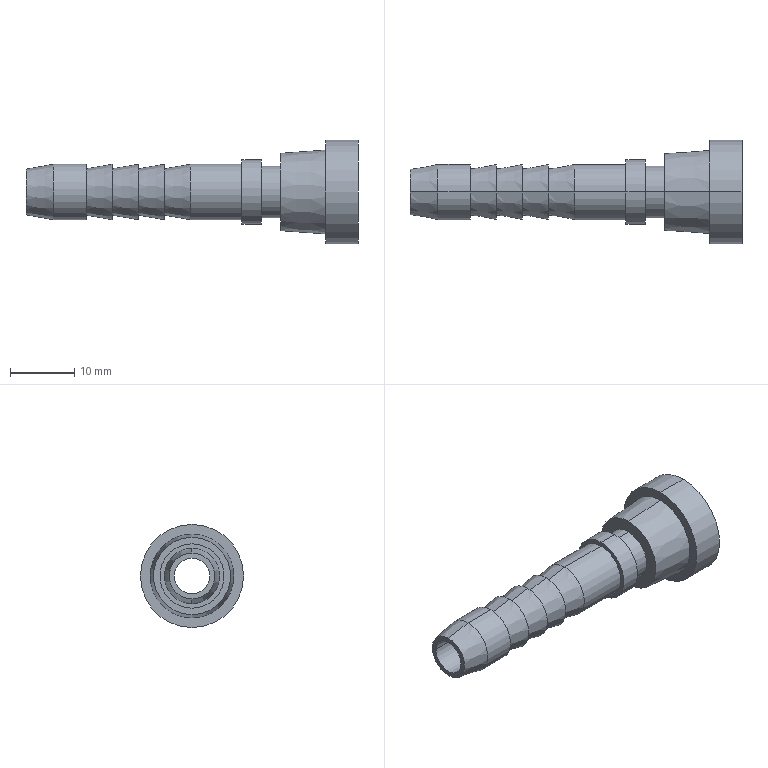Part | SolidWorks | features BaseBody 1 | 1 solid | 34 faces | box 51.5 x 16 x 16 mm | volume 2788 mm3 | cone 12 | cylinder 12 | plane 10 | commonest cylinder face diameters 8.6 x4 5.5 x2 8 x2 10 x2 16 x2
STEP:
#1=CARTESIAN_POINT('',(-12.,0.,-6.));
#2=VERTEX_POINT('',#1);
#3=CARTESIAN_POINT('',(-12.,0.,6.));
#4=VERTEX_POINT('',#3);
#5=CARTESIAN_POINT('',(-12.,0.,0.));
#6=DIRECTION('',(-1.,0.,0.));
#7=DIRECTION('',(0.,0.,-1.));
#8=AXIS2_PLACEMENT_3D('',#5,#6,#7);
#9=CIRCLE('',#8,6.);
#10=EDGE_CURVE('',#2,#4,#9,.T.);
#11=ORIENTED_EDGE('',*,*,#10,.T.);
#12=CARTESIAN_POINT('',(-12.,0.,0.));
#13=DIRECTION('',(-1.,0.,0.));
#14=DIRECTION('',(0.,0.,1.));
#15=AXIS2_PLACEMENT_3D('',#12,#13,#14);
#16=CIRCLE('',#15,6.);
#17=EDGE_CURVE('',#4,#2,#16,.T.);
#18=ORIENTED_EDGE('',*,*,#17,.T.);
#19=EDGE_LOOP('',(#11,#18));
#20=FACE_OUTER_BOUND('',#19,.T.);
#21=CARTESIAN_POINT('',(-12.,0.,4.));
#22=VERTEX_POINT('',#21);
#23=CARTESIAN_POINT('',(-12.,0.,-4.));
#24=VERTEX_POINT('',#23);
#25=CARTESIAN_POINT('',(-12.,0.,0.));
#26=DIRECTION('',(1.,0.,0.));
#27=DIRECTION('',(0.,0.,1.));
#28=AXIS2_PLACEMENT_3D('',#25,#26,#27);
#29=CIRCLE('',#28,4.);
#30=EDGE_CURVE('',#22,#24,#29,.T.);
#31=ORIENTED_EDGE('',*,*,#30,.T.);
#32=CARTESIAN_POINT('',(-12.,0.,0.));
#33=DIRECTION('',(1.,0.,0.));
#34=DIRECTION('',(0.,0.,-1.));
#35=AXIS2_PLACEMENT_3D('',#32,#33,#34);
#36=CIRCLE('',#35,4.);
#37=EDGE_CURVE('',#24,#22,#36,.T.);
#38=ORIENTED_EDGE('',*,*,#37,.T.);
#39=EDGE_LOOP('',(#31,#38));
#40=FACE_BOUND('',#39,.T.);
#41=CARTESIAN_POINT('',(-12.,6.,0.));
#42=DIRECTION('',(-1.,0.,0.));
#43=DIRECTION('',(0.,0.,1.));
#44=AXIS2_PLACEMENT_3D('',#41,#42,#43);
#45=PLANE('',#44);
#46=ADVANCED_FACE('',(#20,#40),#45,.T.);
#47=CARTESIAN_POINT('',(-5.,0.,6.5));
#48=VERTEX_POINT('',#47);
#49=CARTESIAN_POINT('',(-5.,0.,6.5));
#50=DIRECTION('',(-0.9975,0.,-0.07125));
#51=VECTOR('',#50,1000.);
#52=LINE('',#49,#51);
#53=EDGE_CURVE('',#48,#4,#52,.T.);
#54=ORIENTED_EDGE('',*,*,#53,.F.);
#55=CARTESIAN_POINT('',(-5.,0.,-6.5));
#56=VERTEX_POINT('',#55);
#57=CARTESIAN_POINT('',(-5.,0.,0.));
#58=DIRECTION('',(1.,0.,0.));
#59=DIRECTION('',(0.,0.,-1.));
#60=AXIS2_PLACEMENT_3D('',#57,#58,#59);
#61=CIRCLE('',#60,6.5);
#62=EDGE_CURVE('',#56,#48,#61,.T.);
#63=ORIENTED_EDGE('',*,*,#62,.F.);
#64=CARTESIAN_POINT('',(-5.,0.,-6.5));
#65=DIRECTION('',(-0.9975,0.,0.07125));
#66=VECTOR('',#65,1000.);
#67=LINE('',#64,#66);
#68=EDGE_CURVE('',#56,#2,#67,.T.);
#69=ORIENTED_EDGE('',*,*,#68,.T.);
#70=ORIENTED_EDGE('',*,*,#17,.F.);
#71=EDGE_LOOP('',(#54,#63,#69,#70));
#72=FACE_OUTER_BOUND('',#71,.T.);
#73=CARTESIAN_POINT('',(-8.5,0.,0.));
#74=DIRECTION('',(1.,0.,0.));
#75=DIRECTION('',(0.,0.,-1.));
#76=AXIS2_PLACEMENT_3D('',#73,#74,#75);
#77=CONICAL_SURFACE('',#76,6.25,0.07131);
#78=ADVANCED_FACE('',(#72),#77,.T.);
#79=ORIENTED_EDGE('',*,*,#10,.F.);
#80=ORIENTED_EDGE('',*,*,#68,.F.);
#81=CARTESIAN_POINT('',(-5.,0.,0.));
#82=DIRECTION('',(1.,0.,0.));
#83=DIRECTION('',(0.,0.,1.));
#84=AXIS2_PLACEMENT_3D('',#81,#82,#83);
#85=CIRCLE('',#84,6.5);
#86=EDGE_CURVE('',#48,#56,#85,.T.);
#87=ORIENTED_EDGE('',*,*,#86,.F.);
#88=ORIENTED_EDGE('',*,*,#53,.T.);
#89=EDGE_LOOP('',(#79,#80,#87,#88));
#90=FACE_OUTER_BOUND('',#89,.T.);
#91=CARTESIAN_POINT('',(-8.5,0.,0.));
#92=DIRECTION('',(1.,0.,0.));
#93=DIRECTION('',(0.,0.,-1.));
#94=AXIS2_PLACEMENT_3D('',#91,#92,#93);
#95=CONICAL_SURFACE('',#94,6.25,0.07131);
#96=ADVANCED_FACE('',(#90),#95,.T.);
#97=CARTESIAN_POINT('',(-5.,0.,-8.));
#98=VERTEX_POINT('',#97);
#99=CARTESIAN_POINT('',(-5.,0.,8.));
#100=VERTEX_POINT('',#99);
#101=CARTESIAN_POINT('',(-5.,0.,0.));
#102=DIRECTION('',(-1.,0.,0.));
#103=DIRECTION('',(0.,0.,-1.));
#104=AXIS2_PLACEMENT_3D('',#101,#102,#103);
#105=CIRCLE('',#104,8.);
#106=EDGE_CURVE('',#98,#100,#105,.T.);
#107=ORIENTED_EDGE('',*,*,#106,.T.);
#108=CARTESIAN_POINT('',(-5.,0.,0.));
#109=DIRECTION('',(-1.,0.,0.));
#110=DIRECTION('',(0.,0.,1.));
#111=AXIS2_PLACEMENT_3D('',#108,#109,#110);
#112=CIRCLE('',#111,8.);
#113=EDGE_CURVE('',#100,#98,#112,.T.);
#114=ORIENTED_EDGE('',*,*,#113,.T.);
#115=EDGE_LOOP('',(#107,#114));
#116=FACE_OUTER_BOUND('',#115,.T.);
#117=ORIENTED_EDGE('',*,*,#86,.T.);
#118=ORIENTED_EDGE('',*,*,#62,.T.);
#119=EDGE_LOOP('',(#117,#118));
#120=FACE_BOUND('',#119,.T.);
#121=CARTESIAN_POINT('',(-5.,8.,0.));
#122=DIRECTION('',(-1.,0.,0.));
#123=DIRECTION('',(0.,0.,1.));
#124=AXIS2_PLACEMENT_3D('',#121,#122,#123);
#125=PLANE('',#124);
#126=ADVANCED_FACE('',(#116,#120),#125,.T.);
#127=CARTESIAN_POINT('',(0.,0.,8.));
#128=VERTEX_POINT('',#127);
#129=CARTESIAN_POINT('',(0.,0.,8.));
#130=DIRECTION('',(-1.,0.,0.));
#131=VECTOR('',#130,1000.);
#132=LINE('',#129,#131);
#133=EDGE_CURVE('',#128,#100,#132,.T.);
#134=ORIENTED_EDGE('',*,*,#133,.F.);
#135=CARTESIAN_POINT('',(0.,0.,-8.));
#136=VERTEX_POINT('',#135);
#137=CARTESIAN_POINT('',(0.,0.,0.));
#138=DIRECTION('',(1.,0.,0.));
#139=DIRECTION('',(0.,0.,-1.));
#140=AXIS2_PLACEMENT_3D('',#137,#138,#139);
#141=CIRCLE('',#140,8.);
#142=EDGE_CURVE('',#136,#128,#141,.T.);
#143=ORIENTED_EDGE('',*,*,#142,.F.);
#144=CARTESIAN_POINT('',(0.,0.,-8.));
#145=DIRECTION('',(-1.,0.,0.));
#146=VECTOR('',#145,1000.);
#147=LINE('',#144,#146);
#148=EDGE_CURVE('',#136,#98,#147,.T.);
#149=ORIENTED_EDGE('',*,*,#148,.T.);
#150=ORIENTED_EDGE('',*,*,#113,.F.);
#151=EDGE_LOOP('',(#134,#143,#149,#150));
#152=FACE_OUTER_BOUND('',#151,.T.);
#153=CARTESIAN_POINT('',(0.,0.,0.));
#154=DIRECTION('',(1.,0.,0.));
#155=DIRECTION('',(0.,0.,-1.));
#156=AXIS2_PLACEMENT_3D('',#153,#154,#155);
#157=CYLINDRICAL_SURFACE('',#156,8.);
#158=ADVANCED_FACE('',(#152),#157,.T.);
#159=ORIENTED_EDGE('',*,*,#106,.F.);
#160=ORIENTED_EDGE('',*,*,#148,.F.);
#161=CARTESIAN_POINT('',(0.,0.,0.));
#162=DIRECTION('',(1.,0.,0.));
#163=DIRECTION('',(0.,0.,1.));
#164=AXIS2_PLACEMENT_3D('',#161,#162,#163);
#165=CIRCLE('',#164,8.);
#166=EDGE_CURVE('',#128,#136,#165,.T.);
#167=ORIENTED_EDGE('',*,*,#166,.F.);
#168=ORIENTED_EDGE('',*,*,#133,.T.);
#169=EDGE_LOOP('',(#159,#160,#167,#168));
#170=FACE_OUTER_BOUND('',#169,.T.);
#171=CARTESIAN_POINT('',(0.,0.,0.));
#172=DIRECTION('',(1.,0.,0.));
#173=DIRECTION('',(0.,0.,-1.));
#174=AXIS2_PLACEMENT_3D('',#171,#172,#173);
#175=CYLINDRICAL_SURFACE('',#174,8.);
#176=ADVANCED_FACE('',(#170),#175,.T.);
#177=ORIENTED_EDGE('',*,*,#166,.T.);
#178=ORIENTED_EDGE('',*,*,#142,.T.);
#179=EDGE_LOOP('',(#177,#178));
#180=FACE_OUTER_BOUND('',#179,.T.);
#181=CARTESIAN_POINT('',(0.,2.75,0.));
#182=VERTEX_POINT('',#181);
#183=CARTESIAN_POINT('',(0.,-2.75,0.));
#184=VERTEX_POINT('',#183);
#185=CARTESIAN_POINT('',(0.,0.,0.));
#186=DIRECTION('',(-1.,0.,0.));
#187=DIRECTION('',(0.,1.,0.));
#188=AXIS2_PLACEMENT_3D('',#185,#186,#187);
#189=CIRCLE('',#188,2.75);
#190=EDGE_CURVE('',#182,#184,#189,.T.);
#191=ORIENTED_EDGE('',*,*,#190,.T.);
#192=CARTESIAN_POINT('',(0.,0.,0.));
#193=DIRECTION('',(-1.,0.,0.));
#194=DIRECTION('',(0.,-1.,0.));
#195=AXIS2_PLACEMENT_3D('',#192,#193,#194);
#196=CIRCLE('',#195,2.75);
#197=EDGE_CURVE('',#184,#182,#196,.T.);
#198=ORIENTED_EDGE('',*,*,#197,.T.);
#199=EDGE_LOOP('',(#191,#198));
#200=FACE_BOUND('',#199,.T.);
#201=CARTESIAN_POINT('',(0.,2.5,0.));
#202=DIRECTION('',(1.,0.,0.));
#203=DIRECTION('',(0.,1.,0.));
#204=AXIS2_PLACEMENT_3D('',#201,#202,#203);
#205=PLANE('',#204);
#206=ADVANCED_FACE('',(#180,#200),#205,.T.);
#207=CARTESIAN_POINT('',(-51.5,-2.75,0.));
#208=VERTEX_POINT('',#207);
#209=CARTESIAN_POINT('',(-51.5,-2.75,0.));
#210=DIRECTION('',(1.,0.,0.));
#211=VECTOR('',#210,1000.);
#212=LINE('',#209,#211);
#213=EDGE_CURVE('',#208,#184,#212,.T.);
#214=ORIENTED_EDGE('',*,*,#213,.F.);
#215=CARTESIAN_POINT('',(-51.5,2.75,0.));
#216=VERTEX_POINT('',#215);
#217=CARTESIAN_POINT('',(-51.5,0.,0.));
#218=DIRECTION('',(-1.,0.,0.));
#219=DIRECTION('',(0.,-1.,0.));
#220=AXIS2_PLACEMENT_3D('',#217,#218,#219);
#221=CIRCLE('',#220,2.75);
#222=EDGE_CURVE('',#208,#216,#221,.T.);
#223=ORIENTED_EDGE('',*,*,#222,.T.);
#224=CARTESIAN_POINT('',(-51.5,2.75,0.));
#225=DIRECTION('',(1.,0.,0.));
#226=VECTOR('',#225,1000.);
#227=LINE('',#224,#226);
#228=EDGE_CURVE('',#216,#182,#227,.T.);
#229=ORIENTED_EDGE('',*,*,#228,.T.);
#230=ORIENTED_EDGE('',*,*,#197,.F.);
#231=EDGE_LOOP('',(#214,#223,#229,#230));
#232=FACE_OUTER_BOUND('',#231,.T.);
#233=CARTESIAN_POINT('',(-51.5,0.,0.));
#234=DIRECTION('',(-1.,0.,0.));
#235=DIRECTION('',(0.,-1.,0.));
#236=AXIS2_PLACEMENT_3D('',#233,#234,#235);
#237=CYLINDRICAL_SURFACE('',#236,2.75);
#238=ADVANCED_FACE('',(#232),#237,.F.);
#239=ORIENTED_EDGE('',*,*,#228,.F.);
#240=CARTESIAN_POINT('',(-51.5,0.,0.));
#241=DIRECTION('',(-1.,0.,0.));
#242=DIRECTION('',(0.,1.,0.));
#243=AXIS2_PLACEMENT_3D('',#240,#241,#242);
#244=CIRCLE('',#243,2.75);
#245=EDGE_CURVE('',#216,#208,#244,.T.);
#246=ORIENTED_EDGE('',*,*,#245,.T.);
#247=ORIENTED_EDGE('',*,*,#213,.T.);
#248=ORIENTED_EDGE('',*,*,#190,.F.);
#249=EDGE_LOOP('',(#239,#246,#247,#248));
#250=FACE_OUTER_BOUND('',#249,.T.);
#251=CARTESIAN_POINT('',(-51.5,0.,0.));
#252=DIRECTION('',(-1.,0.,0.));
#253=DIRECTION('',(0.,-1.,0.));
#254=AXIS2_PLACEMENT_3D('',#251,#252,#253);
#255=CYLINDRICAL_SURFACE('',#254,2.75);
#256=ADVANCED_FACE('',(#250),#255,.F.);
#257=CARTESIAN_POINT('',(-51.5,0.,3.55));
#258=VERTEX_POINT('',#257);
#259=CARTESIAN_POINT('',(-51.5,0.,-3.55));
#260=VERTEX_POINT('',#259);
#261=CARTESIAN_POINT('',(-51.5,0.,0.));
#262=DIRECTION('',(1.,0.,0.));
#263=DIRECTION('',(0.,0.,1.));
#264=AXIS2_PLACEMENT_3D('',#261,#262,#263);
#265=CIRCLE('',#264,3.55);
#266=EDGE_CURVE('',#258,#260,#265,.T.);
#267=ORIENTED_EDGE('',*,*,#266,.F.);
#268=CARTESIAN_POINT('',(-51.5,0.,0.));
#269=DIRECTION('',(-1.,0.,0.));
#270=DIRECTION('',(0.,0.,1.));
#271=AXIS2_PLACEMENT_3D('',#268,#269,#270);
#272=CIRCLE('',#271,3.55);
#273=EDGE_CURVE('',#258,#260,#272,.T.);
#274=ORIENTED_EDGE('',*,*,#273,.T.);
#275=EDGE_LOOP('',(#267,#274));
#276=FACE_OUTER_BOUND('',#275,.T.);
#277=ORIENTED_EDGE('',*,*,#245,.F.);
#278=ORIENTED_EDGE('',*,*,#222,.F.);
#279=EDGE_LOOP('',(#277,#278));
#280=FACE_BOUND('',#279,.T.);
#281=CARTESIAN_POINT('',(-51.5,3.5,0.));
#282=DIRECTION('',(-1.,0.,0.));
#283=DIRECTION('',(0.,0.,1.));
#284=AXIS2_PLACEMENT_3D('',#281,#282,#283);
#285=PLANE('',#284);
#286=ADVANCED_FACE('',(#276,#280),#285,.T.);
#287=CARTESIAN_POINT('',(-47.169,0.,4.3));
#288=VERTEX_POINT('',#287);
#289=CARTESIAN_POINT('',(-47.169,0.,-4.3));
#290=VERTEX_POINT('',#289);
#291=CARTESIAN_POINT('',(-47.169,0.,0.));
#292=DIRECTION('',(-1.,0.,0.));
#293=DIRECTION('',(0.,0.,1.));
#294=AXIS2_PLACEMENT_3D('',#291,#292,#293);
#295=CIRCLE('',#294,4.3);
#296=EDGE_CURVE('',#288,#290,#295,.T.);
#297=ORIENTED_EDGE('',*,*,#296,.T.);
#298=CARTESIAN_POINT('',(-51.5,0.,-3.55));
#299=DIRECTION('',(0.9853,0.,-0.1706));
#300=VECTOR('',#299,1000.);
#301=LINE('',#298,#300);
#302=EDGE_CURVE('',#260,#290,#301,.T.);
#303=ORIENTED_EDGE('',*,*,#302,.F.);
#304=ORIENTED_EDGE('',*,*,#273,.F.);
#305=CARTESIAN_POINT('',(-51.5,0.,3.55));
#306=DIRECTION('',(0.9853,0.,0.1706));
#307=VECTOR('',#306,1000.);
#308=LINE('',#305,#307);
#309=EDGE_CURVE('',#258,#288,#308,.T.);
#310=ORIENTED_EDGE('',*,*,#309,.T.);
#311=EDGE_LOOP('',(#297,#303,#304,#310));
#312=FACE_OUTER_BOUND('',#311,.T.);
#313=CARTESIAN_POINT('',(-49.335,0.,0.));
#314=DIRECTION('',(1.,0.,0.));
#315=DIRECTION('',(0.,0.,1.));
#316=AXIS2_PLACEMENT_3D('',#313,#314,#315);
#317=CONICAL_SURFACE('',#316,3.925,0.1715);
#318=ADVANCED_FACE('',(#312),#317,.T.);
#319=ORIENTED_EDGE('',*,*,#266,.T.);
#320=ORIENTED_EDGE('',*,*,#302,.T.);
#321=CARTESIAN_POINT('',(-47.169,0.,0.));
#322=DIRECTION('',(1.,0.,0.));
#323=DIRECTION('',(0.,0.,1.));
#324=AXIS2_PLACEMENT_3D('',#321,#322,#323);
#325=CIRCLE('',#324,4.3);
#326=EDGE_CURVE('',#288,#290,#325,.T.);
#327=ORIENTED_EDGE('',*,*,#326,.F.);
#328=ORIENTED_EDGE('',*,*,#309,.F.);
#329=EDGE_LOOP('',(#319,#320,#327,#328));
#330=FACE_OUTER_BOUND('',#329,.T.);
#331=CARTESIAN_POINT('',(-49.335,0.,0.));
#332=DIRECTION('',(1.,0.,0.));
#333=DIRECTION('',(0.,0.,1.));
#334=AXIS2_PLACEMENT_3D('',#331,#332,#333);
#335=CONICAL_SURFACE('',#334,3.925,0.1715);
#336=ADVANCED_FACE('',(#330),#335,.T.);
#337=ORIENTED_EDGE('',*,*,#326,.T.);
#338=CARTESIAN_POINT('',(-42.169,0.,-4.3));
#339=VERTEX_POINT('',#338);
#340=CARTESIAN_POINT('',(-47.169,0.,-4.3));
#341=DIRECTION('',(1.,0.,0.));
#342=VECTOR('',#341,1000.);
#343=LINE('',#340,#342);
#344=EDGE_CURVE('',#290,#339,#343,.T.);
#345=ORIENTED_EDGE('',*,*,#344,.T.);
#346=CARTESIAN_POINT('',(-42.169,0.,4.3));
#347=VERTEX_POINT('',#346);
#348=CARTESIAN_POINT('',(-42.169,0.,0.));
#349=DIRECTION('',(1.,0.,0.));
#350=DIRECTION('',(0.,0.,1.));
#351=AXIS2_PLACEMENT_3D('',#348,#349,#350);
#352=CIRCLE('',#351,4.3);
#353=EDGE_CURVE('',#347,#339,#352,.T.);
#354=ORIENTED_EDGE('',*,*,#353,.F.);
#355=CARTESIAN_POINT('',(-47.169,0.,4.3));
#356=DIRECTION('',(1.,0.,0.));
#357=VECTOR('',#356,1000.);
#358=LINE('',#355,#357);
#359=EDGE_CURVE('',#288,#347,#358,.T.);
#360=ORIENTED_EDGE('',*,*,#359,.F.);
#361=EDGE_LOOP('',(#337,#345,#354,#360));
#362=FACE_OUTER_BOUND('',#361,.T.);
#363=CARTESIAN_POINT('',(-53.175,0.,0.));
#364=DIRECTION('',(1.,0.,0.));
#365=DIRECTION('',(0.,0.,1.));
#366=AXIS2_PLACEMENT_3D('',#363,#364,#365);
#367=CYLINDRICAL_SURFACE('',#366,4.3);
#368=ADVANCED_FACE('',(#362),#367,.T.);
#369=CARTESIAN_POINT('',(-42.169,0.,0.));
#370=DIRECTION('',(-1.,0.,0.));
#371=DIRECTION('',(0.,0.,1.));
#372=AXIS2_PLACEMENT_3D('',#369,#370,#371);
#373=CIRCLE('',#372,4.3);
#374=EDGE_CURVE('',#347,#339,#373,.T.);
#375=ORIENTED_EDGE('',*,*,#374,.T.);
#376=ORIENTED_EDGE('',*,*,#344,.F.);
#377=ORIENTED_EDGE('',*,*,#296,.F.);
#378=ORIENTED_EDGE('',*,*,#359,.T.);
#379=EDGE_LOOP('',(#375,#376,#377,#378));
#380=FACE_OUTER_BOUND('',#379,.T.);
#381=CARTESIAN_POINT('',(-53.175,0.,0.));
#382=DIRECTION('',(1.,0.,0.));
#383=DIRECTION('',(0.,0.,1.));
#384=AXIS2_PLACEMENT_3D('',#381,#382,#383);
#385=CYLINDRICAL_SURFACE('',#384,4.3);
#386=ADVANCED_FACE('',(#380),#385,.T.);
#387=ORIENTED_EDGE('',*,*,#374,.F.);
#388=ORIENTED_EDGE('',*,*,#353,.T.);
#389=EDGE_LOOP('',(#387,#388));
#390=FACE_OUTER_BOUND('',#389,.T.);
#391=CARTESIAN_POINT('',(-42.169,0.,3.6));
#392=VERTEX_POINT('',#391);
#393=CARTESIAN_POINT('',(-42.169,0.,-3.6));
#394=VERTEX_POINT('',#393);
#395=CARTESIAN_POINT('',(-42.169,0.,0.));
#396=DIRECTION('',(1.,0.,0.));
#397=DIRECTION('',(0.,0.,1.));
#398=AXIS2_PLACEMENT_3D('',#395,#396,#397);
#399=CIRCLE('',#398,3.6);
#400=EDGE_CURVE('',#392,#394,#399,.T.);
#401=ORIENTED_EDGE('',*,*,#400,.F.);
#402=CARTESIAN_POINT('',(-42.169,0.,0.));
#403=DIRECTION('',(-1.,0.,0.));
#404=DIRECTION('',(0.,0.,1.));
#405=AXIS2_PLACEMENT_3D('',#402,#403,#404);
#406=CIRCLE('',#405,3.6);
#407=EDGE_CURVE('',#392,#394,#406,.T.);
#408=ORIENTED_EDGE('',*,*,#407,.T.);
#409=EDGE_LOOP('',(#401,#408));
#410=FACE_BOUND('',#409,.T.);
#411=CARTESIAN_POINT('',(-42.169,0.,0.));
#412=DIRECTION('',(1.,0.,0.));
#413=DIRECTION('',(0.,1.,0.));
#414=AXIS2_PLACEMENT_3D('',#411,#412,#413);
#415=PLANE('',#414);
#416=ADVANCED_FACE('',(#390,#410),#415,.T.);
#417=CARTESIAN_POINT('',(-38.127,0.,4.3));
#418=VERTEX_POINT('',#417);
#419=CARTESIAN_POINT('',(-38.127,0.,-4.3));
#420=VERTEX_POINT('',#419);
#421=CARTESIAN_POINT('',(-38.127,0.,0.));
#422=DIRECTION('',(-1.,0.,0.));
#423=DIRECTION('',(0.,0.,1.));
#424=AXIS2_PLACEMENT_3D('',#421,#422,#423);
#425=CIRCLE('',#424,4.3);
#426=EDGE_CURVE('',#418,#420,#425,.T.);
#427=ORIENTED_EDGE('',*,*,#426,.T.);
#428=CARTESIAN_POINT('',(-42.169,0.,-3.6));
#429=DIRECTION('',(0.9853,0.,-0.1706));
#430=VECTOR('',#429,1000.);
#431=LINE('',#428,#430);
#432=EDGE_CURVE('',#394,#420,#431,.T.);
#433=ORIENTED_EDGE('',*,*,#432,.F.);
#434=ORIENTED_EDGE('',*,*,#407,.F.);
#435=CARTESIAN_POINT('',(-42.169,0.,3.6));
#436=DIRECTION('',(0.9853,0.,0.1706));
#437=VECTOR('',#436,1000.);
#438=LINE('',#435,#437);
#439=EDGE_CURVE('',#392,#418,#438,.T.);
#440=ORIENTED_EDGE('',*,*,#439,.T.);
#441=EDGE_LOOP('',(#427,#433,#434,#440));
#442=FACE_OUTER_BOUND('',#441,.T.);
#443=CARTESIAN_POINT('',(-40.148,0.,0.));
#444=DIRECTION('',(1.,0.,0.));
#445=DIRECTION('',(0.,0.,1.));
#446=AXIS2_PLACEMENT_3D('',#443,#444,#445);
#447=CONICAL_SURFACE('',#446,3.95,0.1715);
#448=ADVANCED_FACE('',(#442),#447,.T.);
#449=ORIENTED_EDGE('',*,*,#400,.T.);
#450=ORIENTED_EDGE('',*,*,#432,.T.);
#451=CARTESIAN_POINT('',(-38.127,0.,0.));
#452=DIRECTION('',(1.,0.,0.));
#453=DIRECTION('',(0.,0.,1.));
#454=AXIS2_PLACEMENT_3D('',#451,#452,#453);
#455=CIRCLE('',#454,4.3);
#456=EDGE_CURVE('',#418,#420,#455,.T.);
#457=ORIENTED_EDGE('',*,*,#456,.F.);
#458=ORIENTED_EDGE('',*,*,#439,.F.);
#459=EDGE_LOOP('',(#449,#450,#457,#458));
#460=FACE_OUTER_BOUND('',#459,.T.);
#461=CARTESIAN_POINT('',(-40.148,0.,0.));
#462=DIRECTION('',(1.,0.,0.));
#463=DIRECTION('',(0.,0.,1.));
#464=AXIS2_PLACEMENT_3D('',#461,#462,#463);
#465=CONICAL_SURFACE('',#464,3.95,0.1715);
#466=ADVANCED_FACE('',(#460),#465,.T.);
#467=ORIENTED_EDGE('',*,*,#426,.F.);
#468=ORIENTED_EDGE('',*,*,#456,.T.);
#469=EDGE_LOOP('',(#467,#468));
#470=FACE_OUTER_BOUND('',#469,.T.);
#471=CARTESIAN_POINT('',(-38.127,0.,3.6));
#472=VERTEX_POINT('',#471);
#473=CARTESIAN_POINT('',(-38.127,0.,-3.6));
#474=VERTEX_POINT('',#473);
#475=CARTESIAN_POINT('',(-38.127,0.,0.));
#476=DIRECTION('',(1.,0.,0.));
#477=DIRECTION('',(0.,0.,1.));
#478=AXIS2_PLACEMENT_3D('',#475,#476,#477);
#479=CIRCLE('',#478,3.6);
#480=EDGE_CURVE('',#472,#474,#479,.T.);
#481=ORIENTED_EDGE('',*,*,#480,.F.);
#482=CARTESIAN_POINT('',(-38.127,0.,0.));
#483=DIRECTION('',(-1.,0.,0.));
#484=DIRECTION('',(0.,0.,1.));
#485=AXIS2_PLACEMENT_3D('',#482,#483,#484);
#486=CIRCLE('',#485,3.6);
#487=EDGE_CURVE('',#472,#474,#486,.T.);
#488=ORIENTED_EDGE('',*,*,#487,.T.);
#489=EDGE_LOOP('',(#481,#488));
#490=FACE_BOUND('',#489,.T.);
#491=CARTESIAN_POINT('',(-38.127,0.,0.));
#492=DIRECTION('',(1.,0.,0.));
#493=DIRECTION('',(0.,1.,0.));
#494=AXIS2_PLACEMENT_3D('',#491,#492,#493);
#495=PLANE('',#494);
#496=ADVANCED_FACE('',(#470,#490),#495,.T.);
#497=CARTESIAN_POINT('',(-34.085,0.,4.3));
#498=VERTEX_POINT('',#497);
#499=CARTESIAN_POINT('',(-34.085,0.,-4.3));
#500=VERTEX_POINT('',#499);
#501=CARTESIAN_POINT('',(-34.085,0.,0.));
#502=DIRECTION('',(-1.,0.,0.));
#503=DIRECTION('',(0.,0.,1.));
#504=AXIS2_PLACEMENT_3D('',#501,#502,#503);
#505=CIRCLE('',#504,4.3);
#506=EDGE_CURVE('',#498,#500,#505,.T.);
#507=ORIENTED_EDGE('',*,*,#506,.T.);
#508=CARTESIAN_POINT('',(-38.127,0.,-3.6));
#509=DIRECTION('',(0.9853,0.,-0.1706));
#510=VECTOR('',#509,1000.);
#511=LINE('',#508,#510);
#512=EDGE_CURVE('',#474,#500,#511,.T.);
#513=ORIENTED_EDGE('',*,*,#512,.F.);
#514=ORIENTED_EDGE('',*,*,#487,.F.);
#515=CARTESIAN_POINT('',(-38.127,0.,3.6));
#516=DIRECTION('',(0.9853,0.,0.1706));
#517=VECTOR('',#516,1000.);
#518=LINE('',#515,#517);
#519=EDGE_CURVE('',#472,#498,#518,.T.);
#520=ORIENTED_EDGE('',*,*,#519,.T.);
#521=EDGE_LOOP('',(#507,#513,#514,#520));
#522=FACE_OUTER_BOUND('',#521,.T.);
#523=CARTESIAN_POINT('',(-36.106,0.,0.));
#524=DIRECTION('',(1.,0.,0.));
#525=DIRECTION('',(0.,0.,1.));
#526=AXIS2_PLACEMENT_3D('',#523,#524,#525);
#527=CONICAL_SURFACE('',#526,3.95,0.1715);
#528=ADVANCED_FACE('',(#522),#527,.T.);
#529=ORIENTED_EDGE('',*,*,#480,.T.);
#530=ORIENTED_EDGE('',*,*,#512,.T.);
#531=CARTESIAN_POINT('',(-34.085,0.,0.));
#532=DIRECTION('',(1.,0.,0.));
#533=DIRECTION('',(0.,0.,1.));
#534=AXIS2_PLACEMENT_3D('',#531,#532,#533);
#535=CIRCLE('',#534,4.3);
#536=EDGE_CURVE('',#498,#500,#535,.T.);
#537=ORIENTED_EDGE('',*,*,#536,.F.);
#538=ORIENTED_EDGE('',*,*,#519,.F.);
#539=EDGE_LOOP('',(#529,#530,#537,#538));
#540=FACE_OUTER_BOUND('',#539,.T.);
#541=CARTESIAN_POINT('',(-36.106,0.,0.));
#542=DIRECTION('',(1.,0.,0.));
#543=DIRECTION('',(0.,0.,1.));
#544=AXIS2_PLACEMENT_3D('',#541,#542,#543);
#545=CONICAL_SURFACE('',#544,3.95,0.1715);
#546=ADVANCED_FACE('',(#540),#545,.T.);
#547=ORIENTED_EDGE('',*,*,#506,.F.);
#548=ORIENTED_EDGE('',*,*,#536,.T.);
#549=EDGE_LOOP('',(#547,#548));
#550=FACE_OUTER_BOUND('',#549,.T.);
#551=CARTESIAN_POINT('',(-34.085,0.,3.6));
#552=VERTEX_POINT('',#551);
#553=CARTESIAN_POINT('',(-34.085,0.,-3.6));
#554=VERTEX_POINT('',#553);
#555=CARTESIAN_POINT('',(-34.085,0.,0.));
#556=DIRECTION('',(1.,0.,0.));
#557=DIRECTION('',(0.,0.,1.));
#558=AXIS2_PLACEMENT_3D('',#555,#556,#557);
#559=CIRCLE('',#558,3.6);
#560=EDGE_CURVE('',#552,#554,#559,.T.);
#561=ORIENTED_EDGE('',*,*,#560,.F.);
#562=CARTESIAN_POINT('',(-34.085,0.,0.));
#563=DIRECTION('',(-1.,0.,0.));
#564=DIRECTION('',(0.,0.,1.));
#565=AXIS2_PLACEMENT_3D('',#562,#563,#564);
#566=CIRCLE('',#565,3.6);
#567=EDGE_CURVE('',#552,#554,#566,.T.);
#568=ORIENTED_EDGE('',*,*,#567,.T.);
#569=EDGE_LOOP('',(#561,#568));
#570=FACE_BOUND('',#569,.T.);
#571=CARTESIAN_POINT('',(-34.085,0.,0.));
#572=DIRECTION('',(1.,0.,0.));
#573=DIRECTION('',(0.,1.,0.));
#574=AXIS2_PLACEMENT_3D('',#571,#572,#573);
#575=PLANE('',#574);
#576=ADVANCED_FACE('',(#550,#570),#575,.T.);
#577=CARTESIAN_POINT('',(-30.042,0.,4.3));
#578=VERTEX_POINT('',#577);
#579=CARTESIAN_POINT('',(-30.042,0.,-4.3));
#580=VERTEX_POINT('',#579);
#581=CARTESIAN_POINT('',(-30.042,0.,0.));
#582=DIRECTION('',(-1.,0.,0.));
#583=DIRECTION('',(0.,0.,1.));
#584=AXIS2_PLACEMENT_3D('',#581,#582,#583);
#585=CIRCLE('',#584,4.3);
#586=EDGE_CURVE('',#578,#580,#585,.T.);
#587=ORIENTED_EDGE('',*,*,#586,.T.);
#588=CARTESIAN_POINT('',(-34.085,0.,-3.6));
#589=DIRECTION('',(0.9853,0.,-0.1706));
#590=VECTOR('',#589,1000.);
#591=LINE('',#588,#590);
#592=EDGE_CURVE('',#554,#580,#591,.T.);
#593=ORIENTED_EDGE('',*,*,#592,.F.);
#594=ORIENTED_EDGE('',*,*,#567,.F.);
#595=CARTESIAN_POINT('',(-34.085,0.,3.6));
#596=DIRECTION('',(0.9853,0.,0.1706));
#597=VECTOR('',#596,1000.);
#598=LINE('',#595,#597);
#599=EDGE_CURVE('',#552,#578,#598,.T.);
#600=ORIENTED_EDGE('',*,*,#599,.T.);
#601=EDGE_LOOP('',(#587,#593,#594,#600));
#602=FACE_OUTER_BOUND('',#601,.T.);
#603=CARTESIAN_POINT('',(-32.063,0.,0.));
#604=DIRECTION('',(1.,0.,0.));
#605=DIRECTION('',(0.,0.,1.));
#606=AXIS2_PLACEMENT_3D('',#603,#604,#605);
#607=CONICAL_SURFACE('',#606,3.95,0.1715);
#608=ADVANCED_FACE('',(#602),#607,.T.);
#609=ORIENTED_EDGE('',*,*,#560,.T.);
#610=ORIENTED_EDGE('',*,*,#592,.T.);
#611=CARTESIAN_POINT('',(-30.042,0.,0.));
#612=DIRECTION('',(1.,0.,0.));
#613=DIRECTION('',(0.,0.,1.));
#614=AXIS2_PLACEMENT_3D('',#611,#612,#613);
#615=CIRCLE('',#614,4.3);
#616=EDGE_CURVE('',#578,#580,#615,.T.);
#617=ORIENTED_EDGE('',*,*,#616,.F.);
#618=ORIENTED_EDGE('',*,*,#599,.F.);
#619=EDGE_LOOP('',(#609,#610,#617,#618));
#620=FACE_OUTER_BOUND('',#619,.T.);
#621=CARTESIAN_POINT('',(-32.063,0.,0.));
#622=DIRECTION('',(1.,0.,0.));
#623=DIRECTION('',(0.,0.,1.));
#624=AXIS2_PLACEMENT_3D('',#621,#622,#623);
#625=CONICAL_SURFACE('',#624,3.95,0.1715);
#626=ADVANCED_FACE('',(#620),#625,.T.);
#627=ORIENTED_EDGE('',*,*,#586,.F.);
#628=ORIENTED_EDGE('',*,*,#616,.T.);
#629=EDGE_LOOP('',(#627,#628));
#630=FACE_OUTER_BOUND('',#629,.T.);
#631=CARTESIAN_POINT('',(-30.042,0.,3.6));
#632=VERTEX_POINT('',#631);
#633=CARTESIAN_POINT('',(-30.042,0.,-3.6));
#634=VERTEX_POINT('',#633);
#635=CARTESIAN_POINT('',(-30.042,0.,0.));
#636=DIRECTION('',(1.,0.,0.));
#637=DIRECTION('',(0.,0.,1.));
#638=AXIS2_PLACEMENT_3D('',#635,#636,#637);
#639=CIRCLE('',#638,3.6);
#640=EDGE_CURVE('',#632,#634,#639,.T.);
#641=ORIENTED_EDGE('',*,*,#640,.F.);
#642=CARTESIAN_POINT('',(-30.042,0.,0.));
#643=DIRECTION('',(-1.,0.,0.));
#644=DIRECTION('',(0.,0.,1.));
#645=AXIS2_PLACEMENT_3D('',#642,#643,#644);
#646=CIRCLE('',#645,3.6);
#647=EDGE_CURVE('',#632,#634,#646,.T.);
#648=ORIENTED_EDGE('',*,*,#647,.T.);
#649=EDGE_LOOP('',(#641,#648));
#650=FACE_BOUND('',#649,.T.);
#651=CARTESIAN_POINT('',(-30.042,0.,0.));
#652=DIRECTION('',(1.,0.,0.));
#653=DIRECTION('',(0.,1.,0.));
#654=AXIS2_PLACEMENT_3D('',#651,#652,#653);
#655=PLANE('',#654);
#656=ADVANCED_FACE('',(#630,#650),#655,.T.);
#657=CARTESIAN_POINT('',(-26.,0.,4.3));
#658=VERTEX_POINT('',#657);
#659=CARTESIAN_POINT('',(-26.,0.,-4.3));
#660=VERTEX_POINT('',#659);
#661=CARTESIAN_POINT('',(-26.,0.,0.));
#662=DIRECTION('',(-1.,0.,0.));
#663=DIRECTION('',(0.,0.,1.));
#664=AXIS2_PLACEMENT_3D('',#661,#662,#663);
#665=CIRCLE('',#664,4.3);
#666=EDGE_CURVE('',#658,#660,#665,.T.);
#667=ORIENTED_EDGE('',*,*,#666,.T.);
#668=CARTESIAN_POINT('',(-30.042,0.,-3.6));
#669=DIRECTION('',(0.9853,0.,-0.1706));
#670=VECTOR('',#669,1000.);
#671=LINE('',#668,#670);
#672=EDGE_CURVE('',#634,#660,#671,.T.);
#673=ORIENTED_EDGE('',*,*,#672,.F.);
#674=ORIENTED_EDGE('',*,*,#647,.F.);
#675=CARTESIAN_POINT('',(-30.042,0.,3.6));
#676=DIRECTION('',(0.9853,0.,0.1706));
#677=VECTOR('',#676,1000.);
#678=LINE('',#675,#677);
#679=EDGE_CURVE('',#632,#658,#678,.T.);
#680=ORIENTED_EDGE('',*,*,#679,.T.);
#681=EDGE_LOOP('',(#667,#673,#674,#680));
#682=FACE_OUTER_BOUND('',#681,.T.);
#683=CARTESIAN_POINT('',(-28.021,0.,0.));
#684=DIRECTION('',(1.,0.,0.));
#685=DIRECTION('',(0.,0.,1.));
#686=AXIS2_PLACEMENT_3D('',#683,#684,#685);
#687=CONICAL_SURFACE('',#686,3.95,0.1715);
#688=ADVANCED_FACE('',(#682),#687,.T.);
#689=ORIENTED_EDGE('',*,*,#640,.T.);
#690=ORIENTED_EDGE('',*,*,#672,.T.);
#691=CARTESIAN_POINT('',(-26.,0.,0.));
#692=DIRECTION('',(1.,0.,0.));
#693=DIRECTION('',(0.,0.,1.));
#694=AXIS2_PLACEMENT_3D('',#691,#692,#693);
#695=CIRCLE('',#694,4.3);
#696=EDGE_CURVE('',#658,#660,#695,.T.);
#697=ORIENTED_EDGE('',*,*,#696,.F.);
#698=ORIENTED_EDGE('',*,*,#679,.F.);
#699=EDGE_LOOP('',(#689,#690,#697,#698));
#700=FACE_OUTER_BOUND('',#699,.T.);
#701=CARTESIAN_POINT('',(-28.021,0.,0.));
#702=DIRECTION('',(1.,0.,0.));
#703=DIRECTION('',(0.,0.,1.));
#704=AXIS2_PLACEMENT_3D('',#701,#702,#703);
#705=CONICAL_SURFACE('',#704,3.95,0.1715);
#706=ADVANCED_FACE('',(#700),#705,.T.);
#707=CARTESIAN_POINT('',(-18.,0.,4.3));
#708=VERTEX_POINT('',#707);
#709=CARTESIAN_POINT('',(-26.,0.,4.3));
#710=DIRECTION('',(1.,0.,0.));
#711=VECTOR('',#710,1000.);
#712=LINE('',#709,#711);
#713=EDGE_CURVE('',#658,#708,#712,.T.);
#714=ORIENTED_EDGE('',*,*,#713,.F.);
#715=ORIENTED_EDGE('',*,*,#696,.T.);
#716=CARTESIAN_POINT('',(-18.,0.,-4.3));
#717=VERTEX_POINT('',#716);
#718=CARTESIAN_POINT('',(-26.,0.,-4.3));
#719=DIRECTION('',(1.,0.,0.));
#720=VECTOR('',#719,1000.);
#721=LINE('',#718,#720);
#722=EDGE_CURVE('',#660,#717,#721,.T.);
#723=ORIENTED_EDGE('',*,*,#722,.T.);
#724=CARTESIAN_POINT('',(-18.,0.,0.));
#725=DIRECTION('',(1.,0.,0.));
#726=DIRECTION('',(0.,0.,1.));
#727=AXIS2_PLACEMENT_3D('',#724,#725,#726);
#728=CIRCLE('',#727,4.3);
#729=EDGE_CURVE('',#708,#717,#728,.T.);
#730=ORIENTED_EDGE('',*,*,#729,.F.);
#731=EDGE_LOOP('',(#714,#715,#723,#730));
#732=FACE_OUTER_BOUND('',#731,.T.);
#733=CARTESIAN_POINT('',(-53.175,0.,0.));
#734=DIRECTION('',(1.,0.,0.));
#735=DIRECTION('',(0.,0.,1.));
#736=AXIS2_PLACEMENT_3D('',#733,#734,#735);
#737=CYLINDRICAL_SURFACE('',#736,4.3);
#738=ADVANCED_FACE('',(#732),#737,.T.);
#739=CARTESIAN_POINT('',(-18.,0.,-5.));
#740=VERTEX_POINT('',#739);
#741=CARTESIAN_POINT('',(-18.,0.,5.));
#742=VERTEX_POINT('',#741);
#743=CARTESIAN_POINT('',(-18.,0.,0.));
#744=DIRECTION('',(-1.,0.,0.));
#745=DIRECTION('',(0.,0.,-1.));
#746=AXIS2_PLACEMENT_3D('',#743,#744,#745);
#747=CIRCLE('',#746,5.);
#748=EDGE_CURVE('',#740,#742,#747,.T.);
#749=ORIENTED_EDGE('',*,*,#748,.T.);
#750=CARTESIAN_POINT('',(-18.,0.,0.));
#751=DIRECTION('',(-1.,0.,0.));
#752=DIRECTION('',(0.,0.,1.));
#753=AXIS2_PLACEMENT_3D('',#750,#751,#752);
#754=CIRCLE('',#753,5.);
#755=EDGE_CURVE('',#742,#740,#754,.T.);
#756=ORIENTED_EDGE('',*,*,#755,.T.);
#757=EDGE_LOOP('',(#749,#756));
#758=FACE_OUTER_BOUND('',#757,.T.);
#759=CARTESIAN_POINT('',(-18.,0.,0.));
#760=DIRECTION('',(1.,0.,0.));
#761=DIRECTION('',(0.,0.,-1.));
#762=AXIS2_PLACEMENT_3D('',#759,#760,#761);
#763=CIRCLE('',#762,4.3);
#764=EDGE_CURVE('',#717,#708,#763,.T.);
#765=ORIENTED_EDGE('',*,*,#764,.T.);
#766=ORIENTED_EDGE('',*,*,#729,.T.);
#767=EDGE_LOOP('',(#765,#766));
#768=FACE_BOUND('',#767,.T.);
#769=CARTESIAN_POINT('',(-18.,5.,0.));
#770=DIRECTION('',(-1.,0.,0.));
#771=DIRECTION('',(0.,0.,1.));
#772=AXIS2_PLACEMENT_3D('',#769,#770,#771);
#773=PLANE('',#772);
#774=ADVANCED_FACE('',(#758,#768),#773,.T.);
#775=CARTESIAN_POINT('',(-15.,0.,5.));
#776=VERTEX_POINT('',#775);
#777=CARTESIAN_POINT('',(-15.,0.,5.));
#778=DIRECTION('',(-1.,0.,0.));
#779=VECTOR('',#778,1000.);
#780=LINE('',#777,#779);
#781=EDGE_CURVE('',#776,#742,#780,.T.);
#782=ORIENTED_EDGE('',*,*,#781,.F.);
#783=CARTESIAN_POINT('',(-15.,0.,-5.));
#784=VERTEX_POINT('',#783);
#785=CARTESIAN_POINT('',(-15.,0.,0.));
#786=DIRECTION('',(1.,0.,0.));
#787=DIRECTION('',(0.,0.,-1.));
#788=AXIS2_PLACEMENT_3D('',#785,#786,#787);
#789=CIRCLE('',#788,5.);
#790=EDGE_CURVE('',#784,#776,#789,.T.);
#791=ORIENTED_EDGE('',*,*,#790,.F.);
#792=CARTESIAN_POINT('',(-15.,0.,-5.));
#793=DIRECTION('',(-1.,0.,0.));
#794=VECTOR('',#793,1000.);
#795=LINE('',#792,#794);
#796=EDGE_CURVE('',#784,#740,#795,.T.);
#797=ORIENTED_EDGE('',*,*,#796,.T.);
#798=ORIENTED_EDGE('',*,*,#755,.F.);
#799=EDGE_LOOP('',(#782,#791,#797,#798));
#800=FACE_OUTER_BOUND('',#799,.T.);
#801=CARTESIAN_POINT('',(0.,0.,0.));
#802=DIRECTION('',(1.,0.,0.));
#803=DIRECTION('',(0.,0.,-1.));
#804=AXIS2_PLACEMENT_3D('',#801,#802,#803);
#805=CYLINDRICAL_SURFACE('',#804,5.);
#806=ADVANCED_FACE('',(#800),#805,.T.);
#807=ORIENTED_EDGE('',*,*,#748,.F.);
#808=ORIENTED_EDGE('',*,*,#796,.F.);
#809=CARTESIAN_POINT('',(-15.,0.,0.));
#810=DIRECTION('',(1.,0.,0.));
#811=DIRECTION('',(0.,0.,1.));
#812=AXIS2_PLACEMENT_3D('',#809,#810,#811);
#813=CIRCLE('',#812,5.);
#814=EDGE_CURVE('',#776,#784,#813,.T.);
#815=ORIENTED_EDGE('',*,*,#814,.F.);
#816=ORIENTED_EDGE('',*,*,#781,.T.);
#817=EDGE_LOOP('',(#807,#808,#815,#816));
#818=FACE_OUTER_BOUND('',#817,.T.);
#819=CARTESIAN_POINT('',(0.,0.,0.));
#820=DIRECTION('',(1.,0.,0.));
#821=DIRECTION('',(0.,0.,-1.));
#822=AXIS2_PLACEMENT_3D('',#819,#820,#821);
#823=CYLINDRICAL_SURFACE('',#822,5.);
#824=ADVANCED_FACE('',(#818),#823,.T.);
#825=ORIENTED_EDGE('',*,*,#814,.T.);
#826=ORIENTED_EDGE('',*,*,#790,.T.);
#827=EDGE_LOOP('',(#825,#826));
#828=FACE_OUTER_BOUND('',#827,.T.);
#829=CARTESIAN_POINT('',(-15.,0.,-4.));
#830=VERTEX_POINT('',#829);
#831=CARTESIAN_POINT('',(-15.,0.,4.));
#832=VERTEX_POINT('',#831);
#833=CARTESIAN_POINT('',(-15.,0.,0.));
#834=DIRECTION('',(-1.,0.,0.));
#835=DIRECTION('',(0.,0.,-1.));
#836=AXIS2_PLACEMENT_3D('',#833,#834,#835);
#837=CIRCLE('',#836,4.);
#838=EDGE_CURVE('',#830,#832,#837,.T.);
#839=ORIENTED_EDGE('',*,*,#838,.T.);
#840=CARTESIAN_POINT('',(-15.,0.,0.));
#841=DIRECTION('',(-1.,0.,0.));
#842=DIRECTION('',(0.,0.,1.));
#843=AXIS2_PLACEMENT_3D('',#840,#841,#842);
#844=CIRCLE('',#843,4.);
#845=EDGE_CURVE('',#832,#830,#844,.T.);
#846=ORIENTED_EDGE('',*,*,#845,.T.);
#847=EDGE_LOOP('',(#839,#846));
#848=FACE_BOUND('',#847,.T.);
#849=CARTESIAN_POINT('',(-15.,4.,0.));
#850=DIRECTION('',(1.,0.,0.));
#851=DIRECTION('',(0.,1.,0.));
#852=AXIS2_PLACEMENT_3D('',#849,#850,#851);
#853=PLANE('',#852);
#854=ADVANCED_FACE('',(#828,#848),#853,.T.);
#855=CARTESIAN_POINT('',(-12.,0.,4.));
#856=DIRECTION('',(-1.,0.,0.));
#857=VECTOR('',#856,1000.);
#858=LINE('',#855,#857);
#859=EDGE_CURVE('',#22,#832,#858,.T.);
#860=ORIENTED_EDGE('',*,*,#859,.F.);
#861=ORIENTED_EDGE('',*,*,#37,.F.);
#862=CARTESIAN_POINT('',(-12.,0.,-4.));
#863=DIRECTION('',(-1.,0.,0.));
#864=VECTOR('',#863,1000.);
#865=LINE('',#862,#864);
#866=EDGE_CURVE('',#24,#830,#865,.T.);
#867=ORIENTED_EDGE('',*,*,#866,.T.);
#868=ORIENTED_EDGE('',*,*,#845,.F.);
#869=EDGE_LOOP('',(#860,#861,#867,#868));
#870=FACE_OUTER_BOUND('',#869,.T.);
#871=CARTESIAN_POINT('',(0.,0.,0.));
#872=DIRECTION('',(1.,0.,0.));
#873=DIRECTION('',(0.,0.,-1.));
#874=AXIS2_PLACEMENT_3D('',#871,#872,#873);
#875=CYLINDRICAL_SURFACE('',#874,4.);
#876=ADVANCED_FACE('',(#870),#875,.T.);
#877=ORIENTED_EDGE('',*,*,#838,.F.);
#878=ORIENTED_EDGE('',*,*,#866,.F.);
#879=ORIENTED_EDGE('',*,*,#30,.F.);
#880=ORIENTED_EDGE('',*,*,#859,.T.);
#881=EDGE_LOOP('',(#877,#878,#879,#880));
#882=FACE_OUTER_BOUND('',#881,.T.);
#883=CARTESIAN_POINT('',(0.,0.,0.));
#884=DIRECTION('',(1.,0.,0.));
#885=DIRECTION('',(0.,0.,-1.));
#886=AXIS2_PLACEMENT_3D('',#883,#884,#885);
#887=CYLINDRICAL_SURFACE('',#886,4.);
#888=ADVANCED_FACE('',(#882),#887,.T.);
#889=ORIENTED_EDGE('',*,*,#722,.F.);
#890=ORIENTED_EDGE('',*,*,#666,.F.);
#891=ORIENTED_EDGE('',*,*,#713,.T.);
#892=ORIENTED_EDGE('',*,*,#764,.F.);
#893=EDGE_LOOP('',(#889,#890,#891,#892));
#894=FACE_OUTER_BOUND('',#893,.T.);
#895=CARTESIAN_POINT('',(-53.175,0.,0.));
#896=DIRECTION('',(1.,0.,0.));
#897=DIRECTION('',(0.,0.,1.));
#898=AXIS2_PLACEMENT_3D('',#895,#896,#897);
#899=CYLINDRICAL_SURFACE('',#898,4.3);
#900=ADVANCED_FACE('',(#894),#899,.T.);
#901=CLOSED_SHELL('',(#46,#78,#96,#126,#158,#176,#206,#238,#256,#286,#318,#336,#368,#386,#416,#448,#466,#496,#528,#546,#576,#608,#626,#656,#688,#706,#738,#774,#806,#824,#854,#876,#888,#900));
#902=MANIFOLD_SOLID_BREP('',#901);
#903=CARTESIAN_POINT('',(0.,0.,0.));
#904=DIRECTION('',(0.,0.,1.));
#905=DIRECTION('',(1.,0.,0.));
#906=AXIS2_PLACEMENT_3D('',#903,#904,#905);
#907=(LENGTH_UNIT()NAMED_UNIT(*)SI_UNIT(.MILLI.,.METRE.));
#908=UNCERTAINTY_MEASURE_WITH_UNIT(LENGTH_MEASURE(0.00001),#907,'','');
#909=(NAMED_UNIT(*)PLANE_ANGLE_UNIT()SI_UNIT($,.RADIAN.));
#910=(NAMED_UNIT(*)SI_UNIT($,.STERADIAN.)SOLID_ANGLE_UNIT());
#911=(GEOMETRIC_REPRESENTATION_CONTEXT(3)GLOBAL_UNCERTAINTY_ASSIGNED_CONTEXT((#908))GLOBAL_UNIT_ASSIGNED_CONTEXT((#907,#909,#910))REPRESENTATION_CONTEXT('',''));
#912=ADVANCED_BREP_SHAPE_REPRESENTATION('',(#902,#906),#911);